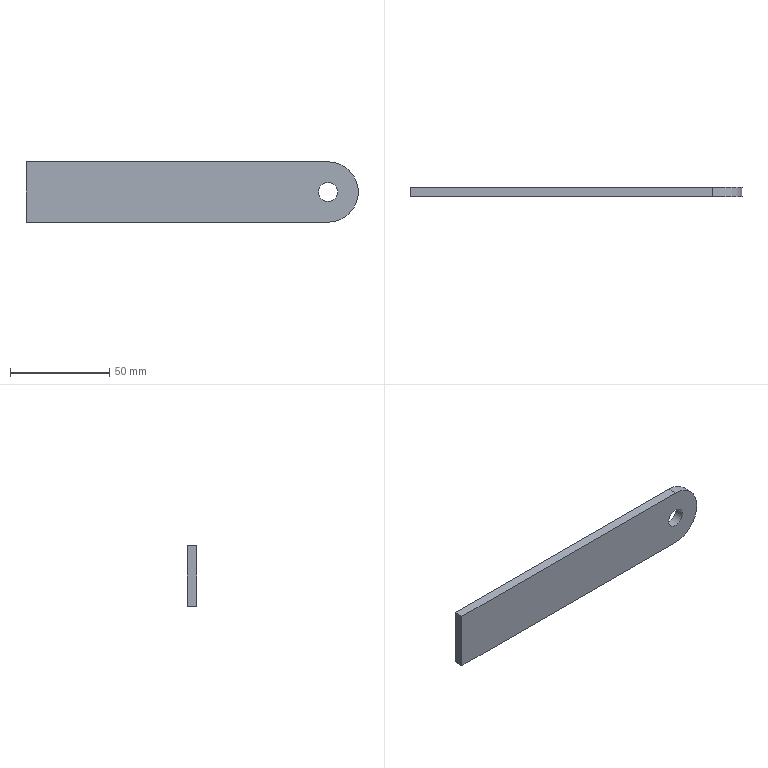Part | NX | features BREP 1 | 1 solid | 8 faces | box 167.64 x 4.763 x 30.48 mm | volume 23512 mm3 | plane 5 | cylinder 3 | commonest cylinder face diameters 9.652 x2 30.48 x1
STEP:
#1=CARTESIAN_POINT('',(0.,0.,15.24));
#2=VERTEX_POINT('',#1);
#3=CARTESIAN_POINT('',(152.4,0.,15.24));
#4=VERTEX_POINT('',#3);
#5=CARTESIAN_POINT('',(0.,0.,15.24));
#6=DIRECTION('',(1.,0.,0.));
#7=VECTOR('',#6,1000.);
#8=LINE('',#5,#7);
#9=EDGE_CURVE('',#2,#4,#8,.T.);
#10=ORIENTED_EDGE('',*,*,#9,.T.);
#11=CARTESIAN_POINT('',(152.4,0.,-15.24));
#12=VERTEX_POINT('',#11);
#13=CARTESIAN_POINT('',(152.4,0.,0.));
#14=DIRECTION('',(0.,1.,0.));
#15=DIRECTION('',(0.,0.,1.));
#16=AXIS2_PLACEMENT_3D('',#13,#14,#15);
#17=CIRCLE('',#16,15.24);
#18=EDGE_CURVE('',#4,#12,#17,.T.);
#19=ORIENTED_EDGE('',*,*,#18,.T.);
#20=CARTESIAN_POINT('',(0.,0.,-15.24));
#21=VERTEX_POINT('',#20);
#22=CARTESIAN_POINT('',(152.4,0.,-15.24));
#23=DIRECTION('',(-1.,0.,0.));
#24=VECTOR('',#23,1000.);
#25=LINE('',#22,#24);
#26=EDGE_CURVE('',#12,#21,#25,.T.);
#27=ORIENTED_EDGE('',*,*,#26,.T.);
#28=CARTESIAN_POINT('',(0.,0.,-15.24));
#29=DIRECTION('',(0.,0.,1.));
#30=VECTOR('',#29,1000.);
#31=LINE('',#28,#30);
#32=EDGE_CURVE('',#21,#2,#31,.T.);
#33=ORIENTED_EDGE('',*,*,#32,.T.);
#34=EDGE_LOOP('',(#10,#19,#27,#33));
#35=FACE_BOUND('',#34,.T.);
#36=CARTESIAN_POINT('',(157.226,0.,0.));
#37=VERTEX_POINT('',#36);
#38=CARTESIAN_POINT('',(147.574,0.,0.));
#39=VERTEX_POINT('',#38);
#40=CARTESIAN_POINT('',(152.4,0.,0.));
#41=DIRECTION('',(0.,1.,0.));
#42=DIRECTION('',(1.,0.,0.));
#43=AXIS2_PLACEMENT_3D('',#40,#41,#42);
#44=CIRCLE('',#43,4.826);
#45=EDGE_CURVE('',#37,#39,#44,.T.);
#46=ORIENTED_EDGE('',*,*,#45,.F.);
#47=CARTESIAN_POINT('',(152.4,0.,0.));
#48=DIRECTION('',(0.,1.,0.));
#49=DIRECTION('',(-1.,0.,0.));
#50=AXIS2_PLACEMENT_3D('',#47,#48,#49);
#51=CIRCLE('',#50,4.826);
#52=EDGE_CURVE('',#39,#37,#51,.T.);
#53=ORIENTED_EDGE('',*,*,#52,.F.);
#54=EDGE_LOOP('',(#46,#53));
#55=FACE_BOUND('',#54,.T.);
#56=CARTESIAN_POINT('',(0.,0.,0.));
#57=DIRECTION('',(0.,1.,0.));
#58=DIRECTION('',(1.,0.,0.));
#59=AXIS2_PLACEMENT_3D('',#56,#57,#58);
#60=PLANE('',#59);
#61=ADVANCED_FACE('',(#35,#55),#60,.T.);
#62=CARTESIAN_POINT('',(0.,-4.763,-15.24));
#63=VERTEX_POINT('',#62);
#64=CARTESIAN_POINT('',(0.,0.,-15.24));
#65=DIRECTION('',(0.,-1.,0.));
#66=VECTOR('',#65,1000.);
#67=LINE('',#64,#66);
#68=EDGE_CURVE('',#21,#63,#67,.T.);
#69=ORIENTED_EDGE('',*,*,#68,.T.);
#70=CARTESIAN_POINT('',(0.,-4.763,15.24));
#71=VERTEX_POINT('',#70);
#72=CARTESIAN_POINT('',(0.,-4.763,-15.24));
#73=DIRECTION('',(0.,0.,1.));
#74=VECTOR('',#73,1000.);
#75=LINE('',#72,#74);
#76=EDGE_CURVE('',#63,#71,#75,.T.);
#77=ORIENTED_EDGE('',*,*,#76,.T.);
#78=CARTESIAN_POINT('',(0.,0.,15.24));
#79=DIRECTION('',(0.,-1.,0.));
#80=VECTOR('',#79,1000.);
#81=LINE('',#78,#80);
#82=EDGE_CURVE('',#2,#71,#81,.T.);
#83=ORIENTED_EDGE('',*,*,#82,.F.);
#84=ORIENTED_EDGE('',*,*,#32,.F.);
#85=EDGE_LOOP('',(#69,#77,#83,#84));
#86=FACE_BOUND('',#85,.T.);
#87=CARTESIAN_POINT('',(0.,-2.381,0.));
#88=DIRECTION('',(-1.,0.,0.));
#89=DIRECTION('',(0.,0.,1.));
#90=AXIS2_PLACEMENT_3D('',#87,#88,#89);
#91=PLANE('',#90);
#92=ADVANCED_FACE('',(#86),#91,.T.);
#93=ORIENTED_EDGE('',*,*,#82,.T.);
#94=CARTESIAN_POINT('',(152.4,-4.763,15.24));
#95=VERTEX_POINT('',#94);
#96=CARTESIAN_POINT('',(0.,-4.763,15.24));
#97=DIRECTION('',(1.,0.,0.));
#98=VECTOR('',#97,1000.);
#99=LINE('',#96,#98);
#100=EDGE_CURVE('',#71,#95,#99,.T.);
#101=ORIENTED_EDGE('',*,*,#100,.T.);
#102=CARTESIAN_POINT('',(152.4,0.,15.24));
#103=DIRECTION('',(0.,-1.,0.));
#104=VECTOR('',#103,1000.);
#105=LINE('',#102,#104);
#106=EDGE_CURVE('',#4,#95,#105,.T.);
#107=ORIENTED_EDGE('',*,*,#106,.F.);
#108=ORIENTED_EDGE('',*,*,#9,.F.);
#109=EDGE_LOOP('',(#93,#101,#107,#108));
#110=FACE_BOUND('',#109,.T.);
#111=CARTESIAN_POINT('',(76.2,-2.381,15.24));
#112=DIRECTION('',(0.,0.,1.));
#113=DIRECTION('',(1.,0.,0.));
#114=AXIS2_PLACEMENT_3D('',#111,#112,#113);
#115=PLANE('',#114);
#116=ADVANCED_FACE('',(#110),#115,.T.);
#117=ORIENTED_EDGE('',*,*,#106,.T.);
#118=CARTESIAN_POINT('',(152.4,-4.763,-15.24));
#119=VERTEX_POINT('',#118);
#120=CARTESIAN_POINT('',(152.4,-4.763,0.));
#121=DIRECTION('',(0.,1.,0.));
#122=DIRECTION('',(0.,0.,1.));
#123=AXIS2_PLACEMENT_3D('',#120,#121,#122);
#124=CIRCLE('',#123,15.24);
#125=EDGE_CURVE('',#95,#119,#124,.T.);
#126=ORIENTED_EDGE('',*,*,#125,.T.);
#127=CARTESIAN_POINT('',(152.4,0.,-15.24));
#128=DIRECTION('',(0.,-1.,0.));
#129=VECTOR('',#128,1000.);
#130=LINE('',#127,#129);
#131=EDGE_CURVE('',#12,#119,#130,.T.);
#132=ORIENTED_EDGE('',*,*,#131,.F.);
#133=ORIENTED_EDGE('',*,*,#18,.F.);
#134=EDGE_LOOP('',(#117,#126,#132,#133));
#135=FACE_BOUND('',#134,.T.);
#136=CARTESIAN_POINT('',(152.4,-2.381,0.));
#137=DIRECTION('',(0.,1.,0.));
#138=DIRECTION('',(0.,0.,1.));
#139=AXIS2_PLACEMENT_3D('',#136,#137,#138);
#140=CYLINDRICAL_SURFACE('',#139,15.24);
#141=ADVANCED_FACE('',(#135),#140,.T.);
#142=ORIENTED_EDGE('',*,*,#131,.T.);
#143=CARTESIAN_POINT('',(152.4,-4.763,-15.24));
#144=DIRECTION('',(-1.,0.,0.));
#145=VECTOR('',#144,1000.);
#146=LINE('',#143,#145);
#147=EDGE_CURVE('',#119,#63,#146,.T.);
#148=ORIENTED_EDGE('',*,*,#147,.T.);
#149=ORIENTED_EDGE('',*,*,#68,.F.);
#150=ORIENTED_EDGE('',*,*,#26,.F.);
#151=EDGE_LOOP('',(#142,#148,#149,#150));
#152=FACE_BOUND('',#151,.T.);
#153=CARTESIAN_POINT('',(76.2,-2.381,-15.24));
#154=DIRECTION('',(0.,0.,-1.));
#155=DIRECTION('',(0.,-1.,0.));
#156=AXIS2_PLACEMENT_3D('',#153,#154,#155);
#157=PLANE('',#156);
#158=ADVANCED_FACE('',(#152),#157,.T.);
#159=ORIENTED_EDGE('',*,*,#147,.F.);
#160=ORIENTED_EDGE('',*,*,#125,.F.);
#161=ORIENTED_EDGE('',*,*,#100,.F.);
#162=ORIENTED_EDGE('',*,*,#76,.F.);
#163=EDGE_LOOP('',(#159,#160,#161,#162));
#164=FACE_BOUND('',#163,.T.);
#165=CARTESIAN_POINT('',(157.226,-4.763,0.));
#166=VERTEX_POINT('',#165);
#167=CARTESIAN_POINT('',(147.574,-4.763,0.));
#168=VERTEX_POINT('',#167);
#169=CARTESIAN_POINT('',(152.4,-4.763,0.));
#170=DIRECTION('',(0.,1.,0.));
#171=DIRECTION('',(1.,0.,0.));
#172=AXIS2_PLACEMENT_3D('',#169,#170,#171);
#173=CIRCLE('',#172,4.826);
#174=EDGE_CURVE('',#166,#168,#173,.T.);
#175=ORIENTED_EDGE('',*,*,#174,.T.);
#176=CARTESIAN_POINT('',(152.4,-4.763,0.));
#177=DIRECTION('',(0.,1.,0.));
#178=DIRECTION('',(-1.,0.,0.));
#179=AXIS2_PLACEMENT_3D('',#176,#177,#178);
#180=CIRCLE('',#179,4.826);
#181=EDGE_CURVE('',#168,#166,#180,.T.);
#182=ORIENTED_EDGE('',*,*,#181,.T.);
#183=EDGE_LOOP('',(#175,#182));
#184=FACE_BOUND('',#183,.T.);
#185=CARTESIAN_POINT('',(0.,-4.763,0.));
#186=DIRECTION('',(0.,1.,0.));
#187=DIRECTION('',(1.,0.,0.));
#188=AXIS2_PLACEMENT_3D('',#185,#186,#187);
#189=PLANE('',#188);
#190=ADVANCED_FACE('',(#164,#184),#189,.F.);
#191=CARTESIAN_POINT('',(157.226,0.,0.));
#192=DIRECTION('',(0.,-1.,0.));
#193=VECTOR('',#192,1000.);
#194=LINE('',#191,#193);
#195=EDGE_CURVE('',#166,#37,#194,.F.);
#196=ORIENTED_EDGE('',*,*,#195,.F.);
#197=ORIENTED_EDGE('',*,*,#181,.F.);
#198=CARTESIAN_POINT('',(147.574,0.,0.));
#199=DIRECTION('',(0.,-1.,0.));
#200=VECTOR('',#199,1000.);
#201=LINE('',#198,#200);
#202=EDGE_CURVE('',#168,#39,#201,.F.);
#203=ORIENTED_EDGE('',*,*,#202,.T.);
#204=ORIENTED_EDGE('',*,*,#52,.T.);
#205=EDGE_LOOP('',(#196,#197,#203,#204));
#206=FACE_BOUND('',#205,.T.);
#207=CARTESIAN_POINT('',(152.4,-2.381,0.));
#208=DIRECTION('',(0.,1.,0.));
#209=DIRECTION('',(-1.,0.,0.));
#210=AXIS2_PLACEMENT_3D('',#207,#208,#209);
#211=CYLINDRICAL_SURFACE('',#210,4.826);
#212=ADVANCED_FACE('',(#206),#211,.F.);
#213=ORIENTED_EDGE('',*,*,#202,.F.);
#214=ORIENTED_EDGE('',*,*,#174,.F.);
#215=ORIENTED_EDGE('',*,*,#195,.T.);
#216=ORIENTED_EDGE('',*,*,#45,.T.);
#217=EDGE_LOOP('',(#213,#214,#215,#216));
#218=FACE_BOUND('',#217,.T.);
#219=CARTESIAN_POINT('',(152.4,-2.381,0.));
#220=DIRECTION('',(0.,1.,0.));
#221=DIRECTION('',(1.,0.,0.));
#222=AXIS2_PLACEMENT_3D('',#219,#220,#221);
#223=CYLINDRICAL_SURFACE('',#222,4.826);
#224=ADVANCED_FACE('',(#218),#223,.F.);
#225=CLOSED_SHELL('',(#61,#92,#116,#141,#158,#190,#212,#224));
#226=MANIFOLD_SOLID_BREP('',#225);
#227=(LENGTH_UNIT()NAMED_UNIT(*)SI_UNIT(.MILLI.,.METRE.));
#228=UNCERTAINTY_MEASURE_WITH_UNIT(LENGTH_MEASURE(0.00001),#227,'','');
#229=(NAMED_UNIT(*)PLANE_ANGLE_UNIT()SI_UNIT($,.RADIAN.));
#230=(NAMED_UNIT(*)SI_UNIT($,.STERADIAN.)SOLID_ANGLE_UNIT());
#231=(GEOMETRIC_REPRESENTATION_CONTEXT(3)GLOBAL_UNCERTAINTY_ASSIGNED_CONTEXT((#228))GLOBAL_UNIT_ASSIGNED_CONTEXT((#227,#229,#230))REPRESENTATION_CONTEXT('',''));
#232=ADVANCED_BREP_SHAPE_REPRESENTATION('',(#226),#231);